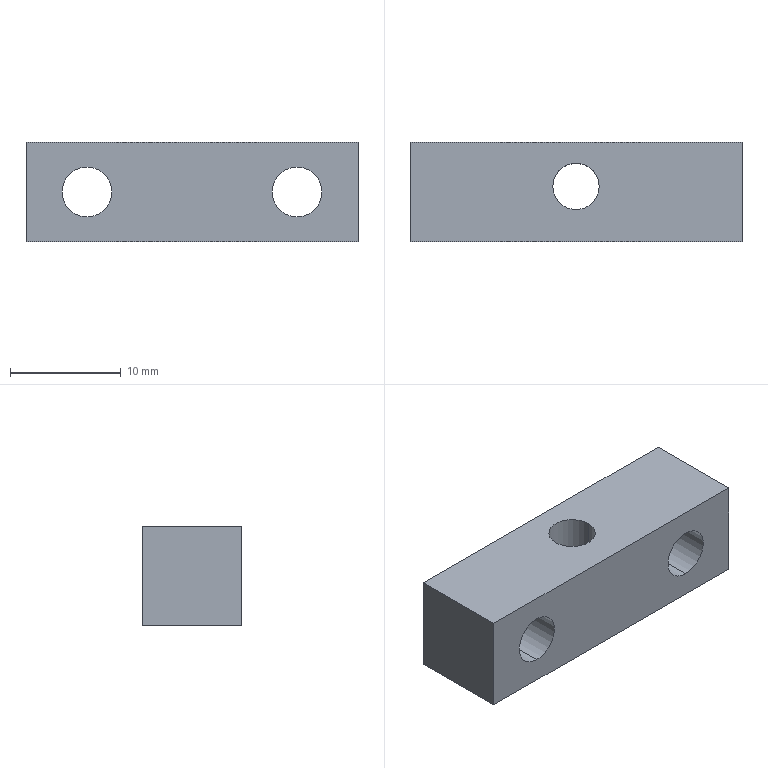Part | STEP file | SceondTSE6-8_Default | 1 solid | 18 faces | box 30 x 9 x 9 mm | volume 1675 mm3 | cylinder 10 | plane 8 | commonest cylinder face diameters 4.5 x4 8 x4 4.2 x2
STEP:
#1=CARTESIAN_POINT('',(0.,0.,0.));
#2=DIRECTION('',(0.,0.,1.));
#3=DIRECTION('',(1.,0.,0.));
#4=AXIS2_PLACEMENT_3D('',#1,#2,#3);
#5=CARTESIAN_POINT('',(2.1,5.,-4.5));
#6=VERTEX_POINT('',#5);
#7=CARTESIAN_POINT('',(2.1,5.,4.5));
#8=VERTEX_POINT('',#7);
#9=CARTESIAN_POINT('',(2.1,5.,4.5));
#10=DIRECTION('',(0.,0.,1.));
#11=VECTOR('',#10,1.);
#12=LINE('',#9,#11);
#13=CARTESIAN_POINT('',(0.,5.,4.5));
#14=DIRECTION('',(0.,0.,1.));
#15=DIRECTION('',(1.,0.,0.));
#16=AXIS2_PLACEMENT_3D('',#13,#14,#15);
#17=CYLINDRICAL_SURFACE('',#16,2.1);
#18=CARTESIAN_POINT('',(6.283,0.));
#19=DIRECTION('',(0.,1.));
#20=VECTOR('',#19,1.);
#21=LINE('',#18,#20);
#22=(GEOMETRIC_REPRESENTATION_CONTEXT(2)PARAMETRIC_REPRESENTATION_CONTEXT()REPRESENTATION_CONTEXT('',''));
#23=DEFINITIONAL_REPRESENTATION('',(#21),#22);
#24=PCURVE('',#17,#23);
#25=CARTESIAN_POINT('',(0.,5.,4.5));
#26=DIRECTION('',(0.,0.,1.));
#27=DIRECTION('',(1.,0.,0.));
#28=AXIS2_PLACEMENT_3D('',#25,#26,#27);
#29=CYLINDRICAL_SURFACE('',#28,2.1);
#30=CARTESIAN_POINT('',(0.,0.));
#31=DIRECTION('',(0.,1.));
#32=VECTOR('',#31,1.);
#33=LINE('',#30,#32);
#34=(GEOMETRIC_REPRESENTATION_CONTEXT(2)PARAMETRIC_REPRESENTATION_CONTEXT()REPRESENTATION_CONTEXT('',''));
#35=DEFINITIONAL_REPRESENTATION('',(#33),#34);
#36=PCURVE('',#29,#35);
#37=SURFACE_CURVE('',#12,(#24,#36),.PCURVE_S1.);
#38=EDGE_CURVE('',#6,#8,#37,.T.);
#39=ORIENTED_EDGE('',*,*,#38,.T.);
#40=CARTESIAN_POINT('',(-2.1,5.,4.5));
#41=VERTEX_POINT('',#40);
#42=CARTESIAN_POINT('',(0.,5.,4.5));
#43=DIRECTION('',(0.,0.,1.));
#44=DIRECTION('',(1.,0.,0.));
#45=AXIS2_PLACEMENT_3D('',#42,#43,#44);
#46=CIRCLE('',#45,2.1);
#47=CARTESIAN_POINT('',(0.,0.));
#48=DIRECTION('',(1.,0.));
#49=VECTOR('',#48,1.);
#50=LINE('',#47,#49);
#51=(GEOMETRIC_REPRESENTATION_CONTEXT(2)PARAMETRIC_REPRESENTATION_CONTEXT()REPRESENTATION_CONTEXT('',''));
#52=DEFINITIONAL_REPRESENTATION('',(#50),#51);
#53=PCURVE('',#17,#52);
#54=CARTESIAN_POINT('',(15.,9.,4.5));
#55=DIRECTION('',(0.,0.,-1.));
#56=DIRECTION('',(-1.,0.,0.));
#57=AXIS2_PLACEMENT_3D('',#54,#55,#56);
#58=PLANE('',#57);
#59=CARTESIAN_POINT('',(12.9,-4.));
#60=CARTESIAN_POINT('',(12.9,-0.3627));
#61=CARTESIAN_POINT('',(16.05,-2.181));
#62=CARTESIAN_POINT('',(19.2,-4.));
#63=CARTESIAN_POINT('',(16.05,-5.819));
#64=CARTESIAN_POINT('',(12.9,-7.637));
#65=CARTESIAN_POINT('',(12.9,-4.));
#66=(BOUNDED_CURVE()B_SPLINE_CURVE(2,(#59,#60,#61,#62,#63,#64,#65),.UNSPECIFIED.,.T.,.F.)B_SPLINE_CURVE_WITH_KNOTS((1,2,2,2,2,1),(-2.094,0.,2.094,4.189,6.283,8.378),.UNSPECIFIED.)CURVE()GEOMETRIC_REPRESENTATION_ITEM()RATIONAL_B_SPLINE_CURVE((1.,0.5,1.,0.5,1.,0.5,1.))REPRESENTATION_ITEM(''));
#67=(GEOMETRIC_REPRESENTATION_CONTEXT(2)PARAMETRIC_REPRESENTATION_CONTEXT()REPRESENTATION_CONTEXT('',''));
#68=DEFINITIONAL_REPRESENTATION('',(#66),#67);
#69=PCURVE('',#58,#68);
#70=SURFACE_CURVE('',#46,(#53,#69),.PCURVE_S1.);
#71=EDGE_CURVE('',#41,#8,#70,.T.);
#72=ORIENTED_EDGE('',*,*,#71,.F.);
#73=CARTESIAN_POINT('',(-2.1,5.,-4.5));
#74=VERTEX_POINT('',#73);
#75=CARTESIAN_POINT('',(-2.1,5.,4.5));
#76=DIRECTION('',(0.,0.,1.));
#77=VECTOR('',#76,1.);
#78=LINE('',#75,#77);
#79=CARTESIAN_POINT('',(3.142,0.));
#80=DIRECTION('',(0.,1.));
#81=VECTOR('',#80,1.);
#82=LINE('',#79,#81);
#83=(GEOMETRIC_REPRESENTATION_CONTEXT(2)PARAMETRIC_REPRESENTATION_CONTEXT()REPRESENTATION_CONTEXT('',''));
#84=DEFINITIONAL_REPRESENTATION('',(#82),#83);
#85=PCURVE('',#17,#84);
#86=CARTESIAN_POINT('',(3.142,0.));
#87=DIRECTION('',(0.,1.));
#88=VECTOR('',#87,1.);
#89=LINE('',#86,#88);
#90=(GEOMETRIC_REPRESENTATION_CONTEXT(2)PARAMETRIC_REPRESENTATION_CONTEXT()REPRESENTATION_CONTEXT('',''));
#91=DEFINITIONAL_REPRESENTATION('',(#89),#90);
#92=PCURVE('',#29,#91);
#93=SURFACE_CURVE('',#78,(#85,#92),.PCURVE_S1.);
#94=EDGE_CURVE('',#74,#41,#93,.T.);
#95=ORIENTED_EDGE('',*,*,#94,.F.);
#96=CARTESIAN_POINT('',(0.,5.,-4.5));
#97=DIRECTION('',(0.,0.,1.));
#98=DIRECTION('',(1.,0.,0.));
#99=AXIS2_PLACEMENT_3D('',#96,#97,#98);
#100=CIRCLE('',#99,2.1);
#101=CARTESIAN_POINT('',(0.,-9.));
#102=DIRECTION('',(1.,0.));
#103=VECTOR('',#102,1.);
#104=LINE('',#101,#103);
#105=(GEOMETRIC_REPRESENTATION_CONTEXT(2)PARAMETRIC_REPRESENTATION_CONTEXT()REPRESENTATION_CONTEXT('',''));
#106=DEFINITIONAL_REPRESENTATION('',(#104),#105);
#107=PCURVE('',#17,#106);
#108=CARTESIAN_POINT('',(15.,9.,-4.5));
#109=DIRECTION('',(0.,0.,1.));
#110=DIRECTION('',(1.,0.,0.));
#111=AXIS2_PLACEMENT_3D('',#108,#109,#110);
#112=PLANE('',#111);
#113=CARTESIAN_POINT('',(-15.,-4.));
#114=DIRECTION('',(1.,0.));
#115=AXIS2_PLACEMENT_2D('',#113,#114);
#116=CIRCLE('',#115,2.1);
#117=(GEOMETRIC_REPRESENTATION_CONTEXT(2)PARAMETRIC_REPRESENTATION_CONTEXT()REPRESENTATION_CONTEXT('',''));
#118=DEFINITIONAL_REPRESENTATION('',(#116),#117);
#119=PCURVE('',#112,#118);
#120=SURFACE_CURVE('',#100,(#107,#119),.PCURVE_S1.);
#121=EDGE_CURVE('',#74,#6,#120,.T.);
#122=ORIENTED_EDGE('',*,*,#121,.T.);
#123=EDGE_LOOP('',(#39,#72,#95,#122));
#124=FACE_BOUND('',#123,.F.);
#125=ADVANCED_FACE('',(#124),#17,.F.);
#126=CARTESIAN_POINT('',(-9.5,4.,4.));
#127=VERTEX_POINT('',#126);
#128=CARTESIAN_POINT('',(-9.5,9.,4.));
#129=VERTEX_POINT('',#128);
#130=CARTESIAN_POINT('',(-9.5,9.,4.));
#131=DIRECTION('',(0.,1.,0.));
#132=VECTOR('',#131,1.);
#133=LINE('',#130,#132);
#134=CARTESIAN_POINT('',(-9.5,9.,0.));
#135=DIRECTION('',(0.,1.,0.));
#136=DIRECTION('',(0.,0.,1.));
#137=AXIS2_PLACEMENT_3D('',#134,#135,#136);
#138=CYLINDRICAL_SURFACE('',#137,4.);
#139=CARTESIAN_POINT('',(6.283,0.));
#140=DIRECTION('',(0.,1.));
#141=VECTOR('',#140,1.);
#142=LINE('',#139,#141);
#143=(GEOMETRIC_REPRESENTATION_CONTEXT(2)PARAMETRIC_REPRESENTATION_CONTEXT()REPRESENTATION_CONTEXT('',''));
#144=DEFINITIONAL_REPRESENTATION('',(#142),#143);
#145=PCURVE('',#138,#144);
#146=CARTESIAN_POINT('',(-9.5,9.,0.));
#147=DIRECTION('',(0.,1.,0.));
#148=DIRECTION('',(0.,0.,1.));
#149=AXIS2_PLACEMENT_3D('',#146,#147,#148);
#150=CYLINDRICAL_SURFACE('',#149,4.);
#151=CARTESIAN_POINT('',(0.,0.));
#152=DIRECTION('',(0.,1.));
#153=VECTOR('',#152,1.);
#154=LINE('',#151,#153);
#155=(GEOMETRIC_REPRESENTATION_CONTEXT(2)PARAMETRIC_REPRESENTATION_CONTEXT()REPRESENTATION_CONTEXT('',''));
#156=DEFINITIONAL_REPRESENTATION('',(#154),#155);
#157=PCURVE('',#150,#156);
#158=SURFACE_CURVE('',#133,(#145,#157),.PCURVE_S1.);
#159=EDGE_CURVE('',#127,#129,#158,.T.);
#160=ORIENTED_EDGE('',*,*,#159,.T.);
#161=CARTESIAN_POINT('',(-9.5,9.,-4.));
#162=VERTEX_POINT('',#161);
#163=CARTESIAN_POINT('',(-9.5,9.,0.));
#164=DIRECTION('',(0.,1.,0.));
#165=DIRECTION('',(0.,0.,1.));
#166=AXIS2_PLACEMENT_3D('',#163,#164,#165);
#167=CIRCLE('',#166,4.);
#168=CARTESIAN_POINT('',(0.,0.));
#169=DIRECTION('',(1.,0.));
#170=VECTOR('',#169,1.);
#171=LINE('',#168,#170);
#172=(GEOMETRIC_REPRESENTATION_CONTEXT(2)PARAMETRIC_REPRESENTATION_CONTEXT()REPRESENTATION_CONTEXT('',''));
#173=DEFINITIONAL_REPRESENTATION('',(#171),#172);
#174=PCURVE('',#138,#173);
#175=CARTESIAN_POINT('',(0.,9.,0.));
#176=DIRECTION('',(0.,1.,0.));
#177=DIRECTION('',(0.,0.,1.));
#178=AXIS2_PLACEMENT_3D('',#175,#176,#177);
#179=PLANE('',#178);
#180=CARTESIAN_POINT('',(0.,-9.5));
#181=DIRECTION('',(1.,0.));
#182=AXIS2_PLACEMENT_2D('',#180,#181);
#183=CIRCLE('',#182,4.);
#184=(GEOMETRIC_REPRESENTATION_CONTEXT(2)PARAMETRIC_REPRESENTATION_CONTEXT()REPRESENTATION_CONTEXT('',''));
#185=DEFINITIONAL_REPRESENTATION('',(#183),#184);
#186=PCURVE('',#179,#185);
#187=SURFACE_CURVE('',#167,(#174,#186),.PCURVE_S1.);
#188=EDGE_CURVE('',#162,#129,#187,.T.);
#189=ORIENTED_EDGE('',*,*,#188,.F.);
#190=CARTESIAN_POINT('',(-9.5,4.,-4.));
#191=VERTEX_POINT('',#190);
#192=CARTESIAN_POINT('',(-9.5,9.,-4.));
#193=DIRECTION('',(0.,1.,0.));
#194=VECTOR('',#193,1.);
#195=LINE('',#192,#194);
#196=CARTESIAN_POINT('',(3.142,0.));
#197=DIRECTION('',(0.,1.));
#198=VECTOR('',#197,1.);
#199=LINE('',#196,#198);
#200=(GEOMETRIC_REPRESENTATION_CONTEXT(2)PARAMETRIC_REPRESENTATION_CONTEXT()REPRESENTATION_CONTEXT('',''));
#201=DEFINITIONAL_REPRESENTATION('',(#199),#200);
#202=PCURVE('',#138,#201);
#203=CARTESIAN_POINT('',(3.142,0.));
#204=DIRECTION('',(0.,1.));
#205=VECTOR('',#204,1.);
#206=LINE('',#203,#205);
#207=(GEOMETRIC_REPRESENTATION_CONTEXT(2)PARAMETRIC_REPRESENTATION_CONTEXT()REPRESENTATION_CONTEXT('',''));
#208=DEFINITIONAL_REPRESENTATION('',(#206),#207);
#209=PCURVE('',#150,#208);
#210=SURFACE_CURVE('',#195,(#202,#209),.PCURVE_S1.);
#211=EDGE_CURVE('',#191,#162,#210,.T.);
#212=ORIENTED_EDGE('',*,*,#211,.F.);
#213=CARTESIAN_POINT('',(-9.5,4.,0.));
#214=DIRECTION('',(0.,1.,0.));
#215=DIRECTION('',(0.,0.,1.));
#216=AXIS2_PLACEMENT_3D('',#213,#214,#215);
#217=CIRCLE('',#216,4.);
#218=CARTESIAN_POINT('',(0.,-5.));
#219=DIRECTION('',(1.,0.));
#220=VECTOR('',#219,1.);
#221=LINE('',#218,#220);
#222=(GEOMETRIC_REPRESENTATION_CONTEXT(2)PARAMETRIC_REPRESENTATION_CONTEXT()REPRESENTATION_CONTEXT('',''));
#223=DEFINITIONAL_REPRESENTATION('',(#221),#222);
#224=PCURVE('',#138,#223);
#225=CARTESIAN_POINT('',(-7.25,4.,0.));
#226=DIRECTION('',(0.,-1.,0.));
#227=DIRECTION('',(0.,0.,-1.));
#228=AXIS2_PLACEMENT_3D('',#225,#226,#227);
#229=PLANE('',#228);
#230=CARTESIAN_POINT('',(-4.,-2.25));
#231=CARTESIAN_POINT('',(-4.,4.678));
#232=CARTESIAN_POINT('',(2.,1.214));
#233=CARTESIAN_POINT('',(8.,-2.25));
#234=CARTESIAN_POINT('',(2.,-5.714));
#235=CARTESIAN_POINT('',(-4.,-9.178));
#236=CARTESIAN_POINT('',(-4.,-2.25));
#237=(BOUNDED_CURVE()B_SPLINE_CURVE(2,(#230,#231,#232,#233,#234,#235,#236),.UNSPECIFIED.,.T.,.F.)B_SPLINE_CURVE_WITH_KNOTS((1,2,2,2,2,1),(-2.094,0.,2.094,4.189,6.283,8.378),.UNSPECIFIED.)CURVE()GEOMETRIC_REPRESENTATION_ITEM()RATIONAL_B_SPLINE_CURVE((1.,0.5,1.,0.5,1.,0.5,1.))REPRESENTATION_ITEM(''));
#238=(GEOMETRIC_REPRESENTATION_CONTEXT(2)PARAMETRIC_REPRESENTATION_CONTEXT()REPRESENTATION_CONTEXT('',''));
#239=DEFINITIONAL_REPRESENTATION('',(#237),#238);
#240=PCURVE('',#229,#239);
#241=SURFACE_CURVE('',#217,(#224,#240),.PCURVE_S1.);
#242=EDGE_CURVE('',#191,#127,#241,.T.);
#243=ORIENTED_EDGE('',*,*,#242,.T.);
#244=EDGE_LOOP('',(#160,#189,#212,#243));
#245=FACE_BOUND('',#244,.F.);
#246=ADVANCED_FACE('',(#245),#138,.F.);
#247=CARTESIAN_POINT('',(-9.5,0.,2.25));
#248=VERTEX_POINT('',#247);
#249=CARTESIAN_POINT('',(-9.5,4.,2.25));
#250=VERTEX_POINT('',#249);
#251=CARTESIAN_POINT('',(-9.5,9.,2.25));
#252=DIRECTION('',(0.,1.,0.));
#253=VECTOR('',#252,1.);
#254=LINE('',#251,#253);
#255=CARTESIAN_POINT('',(-9.5,9.,0.));
#256=DIRECTION('',(0.,1.,0.));
#257=DIRECTION('',(0.,0.,1.));
#258=AXIS2_PLACEMENT_3D('',#255,#256,#257);
#259=CYLINDRICAL_SURFACE('',#258,2.25);
#260=CARTESIAN_POINT('',(6.283,0.));
#261=DIRECTION('',(0.,1.));
#262=VECTOR('',#261,1.);
#263=LINE('',#260,#262);
#264=(GEOMETRIC_REPRESENTATION_CONTEXT(2)PARAMETRIC_REPRESENTATION_CONTEXT()REPRESENTATION_CONTEXT('',''));
#265=DEFINITIONAL_REPRESENTATION('',(#263),#264);
#266=PCURVE('',#259,#265);
#267=CARTESIAN_POINT('',(-9.5,9.,0.));
#268=DIRECTION('',(0.,1.,0.));
#269=DIRECTION('',(0.,0.,1.));
#270=AXIS2_PLACEMENT_3D('',#267,#268,#269);
#271=CYLINDRICAL_SURFACE('',#270,2.25);
#272=CARTESIAN_POINT('',(0.,0.));
#273=DIRECTION('',(0.,1.));
#274=VECTOR('',#273,1.);
#275=LINE('',#272,#274);
#276=(GEOMETRIC_REPRESENTATION_CONTEXT(2)PARAMETRIC_REPRESENTATION_CONTEXT()REPRESENTATION_CONTEXT('',''));
#277=DEFINITIONAL_REPRESENTATION('',(#275),#276);
#278=PCURVE('',#271,#277);
#279=SURFACE_CURVE('',#254,(#266,#278),.PCURVE_S1.);
#280=EDGE_CURVE('',#248,#250,#279,.T.);
#281=ORIENTED_EDGE('',*,*,#280,.T.);
#282=CARTESIAN_POINT('',(-9.5,4.,-2.25));
#283=VERTEX_POINT('',#282);
#284=CARTESIAN_POINT('',(-9.5,4.,0.));
#285=DIRECTION('',(0.,1.,0.));
#286=DIRECTION('',(0.,0.,1.));
#287=AXIS2_PLACEMENT_3D('',#284,#285,#286);
#288=CIRCLE('',#287,2.25);
#289=CARTESIAN_POINT('',(0.,-5.));
#290=DIRECTION('',(1.,0.));
#291=VECTOR('',#290,1.);
#292=LINE('',#289,#291);
#293=(GEOMETRIC_REPRESENTATION_CONTEXT(2)PARAMETRIC_REPRESENTATION_CONTEXT()REPRESENTATION_CONTEXT('',''));
#294=DEFINITIONAL_REPRESENTATION('',(#292),#293);
#295=PCURVE('',#259,#294);
#296=CARTESIAN_POINT('',(-2.25,-2.25));
#297=CARTESIAN_POINT('',(-2.25,1.647));
#298=CARTESIAN_POINT('',(1.125,-0.3014));
#299=CARTESIAN_POINT('',(4.5,-2.25));
#300=CARTESIAN_POINT('',(1.125,-4.199));
#301=CARTESIAN_POINT('',(-2.25,-6.147));
#302=CARTESIAN_POINT('',(-2.25,-2.25));
#303=(BOUNDED_CURVE()B_SPLINE_CURVE(2,(#296,#297,#298,#299,#300,#301,#302),.UNSPECIFIED.,.T.,.F.)B_SPLINE_CURVE_WITH_KNOTS((1,2,2,2,2,1),(-2.094,0.,2.094,4.189,6.283,8.378),.UNSPECIFIED.)CURVE()GEOMETRIC_REPRESENTATION_ITEM()RATIONAL_B_SPLINE_CURVE((1.,0.5,1.,0.5,1.,0.5,1.))REPRESENTATION_ITEM(''));
#304=(GEOMETRIC_REPRESENTATION_CONTEXT(2)PARAMETRIC_REPRESENTATION_CONTEXT()REPRESENTATION_CONTEXT('',''));
#305=DEFINITIONAL_REPRESENTATION('',(#303),#304);
#306=PCURVE('',#229,#305);
#307=SURFACE_CURVE('',#288,(#295,#306),.PCURVE_S1.);
#308=EDGE_CURVE('',#283,#250,#307,.T.);
#309=ORIENTED_EDGE('',*,*,#308,.F.);
#310=CARTESIAN_POINT('',(-9.5,0.,-2.25));
#311=VERTEX_POINT('',#310);
#312=CARTESIAN_POINT('',(-9.5,9.,-2.25));
#313=DIRECTION('',(0.,1.,0.));
#314=VECTOR('',#313,1.);
#315=LINE('',#312,#314);
#316=CARTESIAN_POINT('',(3.142,0.));
#317=DIRECTION('',(0.,1.));
#318=VECTOR('',#317,1.);
#319=LINE('',#316,#318);
#320=(GEOMETRIC_REPRESENTATION_CONTEXT(2)PARAMETRIC_REPRESENTATION_CONTEXT()REPRESENTATION_CONTEXT('',''));
#321=DEFINITIONAL_REPRESENTATION('',(#319),#320);
#322=PCURVE('',#259,#321);
#323=CARTESIAN_POINT('',(3.142,0.));
#324=DIRECTION('',(0.,1.));
#325=VECTOR('',#324,1.);
#326=LINE('',#323,#325);
#327=(GEOMETRIC_REPRESENTATION_CONTEXT(2)PARAMETRIC_REPRESENTATION_CONTEXT()REPRESENTATION_CONTEXT('',''));
#328=DEFINITIONAL_REPRESENTATION('',(#326),#327);
#329=PCURVE('',#271,#328);
#330=SURFACE_CURVE('',#315,(#322,#329),.PCURVE_S1.);
#331=EDGE_CURVE('',#311,#283,#330,.T.);
#332=ORIENTED_EDGE('',*,*,#331,.F.);
#333=CARTESIAN_POINT('',(-9.5,0.,0.));
#334=DIRECTION('',(0.,1.,0.));
#335=DIRECTION('',(0.,0.,1.));
#336=AXIS2_PLACEMENT_3D('',#333,#334,#335);
#337=CIRCLE('',#336,2.25);
#338=CARTESIAN_POINT('',(0.,-9.));
#339=DIRECTION('',(1.,0.));
#340=VECTOR('',#339,1.);
#341=LINE('',#338,#340);
#342=(GEOMETRIC_REPRESENTATION_CONTEXT(2)PARAMETRIC_REPRESENTATION_CONTEXT()REPRESENTATION_CONTEXT('',''));
#343=DEFINITIONAL_REPRESENTATION('',(#341),#342);
#344=PCURVE('',#259,#343);
#345=CARTESIAN_POINT('',(0.,0.,0.));
#346=DIRECTION('',(0.,1.,0.));
#347=DIRECTION('',(0.,0.,1.));
#348=AXIS2_PLACEMENT_3D('',#345,#346,#347);
#349=PLANE('',#348);
#350=CARTESIAN_POINT('',(0.,-9.5));
#351=DIRECTION('',(1.,0.));
#352=AXIS2_PLACEMENT_2D('',#350,#351);
#353=CIRCLE('',#352,2.25);
#354=(GEOMETRIC_REPRESENTATION_CONTEXT(2)PARAMETRIC_REPRESENTATION_CONTEXT()REPRESENTATION_CONTEXT('',''));
#355=DEFINITIONAL_REPRESENTATION('',(#353),#354);
#356=PCURVE('',#349,#355);
#357=SURFACE_CURVE('',#337,(#344,#356),.PCURVE_S1.);
#358=EDGE_CURVE('',#311,#248,#357,.T.);
#359=ORIENTED_EDGE('',*,*,#358,.T.);
#360=EDGE_LOOP('',(#281,#309,#332,#359));
#361=FACE_BOUND('',#360,.F.);
#362=ADVANCED_FACE('',(#361),#259,.F.);
#363=CARTESIAN_POINT('',(9.5,4.,4.));
#364=VERTEX_POINT('',#363);
#365=CARTESIAN_POINT('',(9.5,9.,4.));
#366=VERTEX_POINT('',#365);
#367=CARTESIAN_POINT('',(9.5,9.,4.));
#368=DIRECTION('',(0.,1.,0.));
#369=VECTOR('',#368,1.);
#370=LINE('',#367,#369);
#371=CARTESIAN_POINT('',(9.5,9.,0.));
#372=DIRECTION('',(0.,1.,0.));
#373=DIRECTION('',(0.,0.,1.));
#374=AXIS2_PLACEMENT_3D('',#371,#372,#373);
#375=CYLINDRICAL_SURFACE('',#374,4.);
#376=CARTESIAN_POINT('',(6.283,0.));
#377=DIRECTION('',(0.,1.));
#378=VECTOR('',#377,1.);
#379=LINE('',#376,#378);
#380=(GEOMETRIC_REPRESENTATION_CONTEXT(2)PARAMETRIC_REPRESENTATION_CONTEXT()REPRESENTATION_CONTEXT('',''));
#381=DEFINITIONAL_REPRESENTATION('',(#379),#380);
#382=PCURVE('',#375,#381);
#383=CARTESIAN_POINT('',(9.5,9.,0.));
#384=DIRECTION('',(0.,1.,0.));
#385=DIRECTION('',(0.,0.,1.));
#386=AXIS2_PLACEMENT_3D('',#383,#384,#385);
#387=CYLINDRICAL_SURFACE('',#386,4.);
#388=CARTESIAN_POINT('',(0.,0.));
#389=DIRECTION('',(0.,1.));
#390=VECTOR('',#389,1.);
#391=LINE('',#388,#390);
#392=(GEOMETRIC_REPRESENTATION_CONTEXT(2)PARAMETRIC_REPRESENTATION_CONTEXT()REPRESENTATION_CONTEXT('',''));
#393=DEFINITIONAL_REPRESENTATION('',(#391),#392);
#394=PCURVE('',#387,#393);
#395=SURFACE_CURVE('',#370,(#382,#394),.PCURVE_S1.);
#396=EDGE_CURVE('',#364,#366,#395,.T.);
#397=ORIENTED_EDGE('',*,*,#396,.T.);
#398=CARTESIAN_POINT('',(9.5,9.,-4.));
#399=VERTEX_POINT('',#398);
#400=CARTESIAN_POINT('',(9.5,9.,0.));
#401=DIRECTION('',(0.,1.,0.));
#402=DIRECTION('',(0.,0.,1.));
#403=AXIS2_PLACEMENT_3D('',#400,#401,#402);
#404=CIRCLE('',#403,4.);
#405=CARTESIAN_POINT('',(0.,0.));
#406=DIRECTION('',(1.,0.));
#407=VECTOR('',#406,1.);
#408=LINE('',#405,#407);
#409=(GEOMETRIC_REPRESENTATION_CONTEXT(2)PARAMETRIC_REPRESENTATION_CONTEXT()REPRESENTATION_CONTEXT('',''));
#410=DEFINITIONAL_REPRESENTATION('',(#408),#409);
#411=PCURVE('',#375,#410);
#412=CARTESIAN_POINT('',(0.,9.5));
#413=DIRECTION('',(1.,0.));
#414=AXIS2_PLACEMENT_2D('',#412,#413);
#415=CIRCLE('',#414,4.);
#416=(GEOMETRIC_REPRESENTATION_CONTEXT(2)PARAMETRIC_REPRESENTATION_CONTEXT()REPRESENTATION_CONTEXT('',''));
#417=DEFINITIONAL_REPRESENTATION('',(#415),#416);
#418=PCURVE('',#179,#417);
#419=SURFACE_CURVE('',#404,(#411,#418),.PCURVE_S1.);
#420=EDGE_CURVE('',#399,#366,#419,.T.);
#421=ORIENTED_EDGE('',*,*,#420,.F.);
#422=CARTESIAN_POINT('',(9.5,4.,-4.));
#423=VERTEX_POINT('',#422);
#424=CARTESIAN_POINT('',(9.5,9.,-4.));
#425=DIRECTION('',(0.,1.,0.));
#426=VECTOR('',#425,1.);
#427=LINE('',#424,#426);
#428=CARTESIAN_POINT('',(3.142,0.));
#429=DIRECTION('',(0.,1.));
#430=VECTOR('',#429,1.);
#431=LINE('',#428,#430);
#432=(GEOMETRIC_REPRESENTATION_CONTEXT(2)PARAMETRIC_REPRESENTATION_CONTEXT()REPRESENTATION_CONTEXT('',''));
#433=DEFINITIONAL_REPRESENTATION('',(#431),#432);
#434=PCURVE('',#375,#433);
#435=CARTESIAN_POINT('',(3.142,0.));
#436=DIRECTION('',(0.,1.));
#437=VECTOR('',#436,1.);
#438=LINE('',#435,#437);
#439=(GEOMETRIC_REPRESENTATION_CONTEXT(2)PARAMETRIC_REPRESENTATION_CONTEXT()REPRESENTATION_CONTEXT('',''));
#440=DEFINITIONAL_REPRESENTATION('',(#438),#439);
#441=PCURVE('',#387,#440);
#442=SURFACE_CURVE('',#427,(#434,#441),.PCURVE_S1.);
#443=EDGE_CURVE('',#423,#399,#442,.T.);
#444=ORIENTED_EDGE('',*,*,#443,.F.);
#445=CARTESIAN_POINT('',(9.5,4.,0.));
#446=DIRECTION('',(0.,1.,0.));
#447=DIRECTION('',(0.,0.,1.));
#448=AXIS2_PLACEMENT_3D('',#445,#446,#447);
#449=CIRCLE('',#448,4.);
#450=CARTESIAN_POINT('',(0.,-5.));
#451=DIRECTION('',(1.,0.));
#452=VECTOR('',#451,1.);
#453=LINE('',#450,#452);
#454=(GEOMETRIC_REPRESENTATION_CONTEXT(2)PARAMETRIC_REPRESENTATION_CONTEXT()REPRESENTATION_CONTEXT('',''));
#455=DEFINITIONAL_REPRESENTATION('',(#453),#454);
#456=PCURVE('',#375,#455);
#457=CARTESIAN_POINT('',(11.75,4.,0.));
#458=DIRECTION('',(0.,-1.,0.));
#459=DIRECTION('',(0.,0.,-1.));
#460=AXIS2_PLACEMENT_3D('',#457,#458,#459);
#461=PLANE('',#460);
#462=CARTESIAN_POINT('',(-4.,-2.25));
#463=CARTESIAN_POINT('',(-4.,4.678));
#464=CARTESIAN_POINT('',(2.,1.214));
#465=CARTESIAN_POINT('',(8.,-2.25));
#466=CARTESIAN_POINT('',(2.,-5.714));
#467=CARTESIAN_POINT('',(-4.,-9.178));
#468=CARTESIAN_POINT('',(-4.,-2.25));
#469=(BOUNDED_CURVE()B_SPLINE_CURVE(2,(#462,#463,#464,#465,#466,#467,#468),.UNSPECIFIED.,.T.,.F.)B_SPLINE_CURVE_WITH_KNOTS((1,2,2,2,2,1),(-2.094,0.,2.094,4.189,6.283,8.378),.UNSPECIFIED.)CURVE()GEOMETRIC_REPRESENTATION_ITEM()RATIONAL_B_SPLINE_CURVE((1.,0.5,1.,0.5,1.,0.5,1.))REPRESENTATION_ITEM(''));
#470=(GEOMETRIC_REPRESENTATION_CONTEXT(2)PARAMETRIC_REPRESENTATION_CONTEXT()REPRESENTATION_CONTEXT('',''));
#471=DEFINITIONAL_REPRESENTATION('',(#469),#470);
#472=PCURVE('',#461,#471);
#473=SURFACE_CURVE('',#449,(#456,#472),.PCURVE_S1.);
#474=EDGE_CURVE('',#423,#364,#473,.T.);
#475=ORIENTED_EDGE('',*,*,#474,.T.);
#476=EDGE_LOOP('',(#397,#421,#444,#475));
#477=FACE_BOUND('',#476,.F.);
#478=ADVANCED_FACE('',(#477),#375,.F.);
#479=CARTESIAN_POINT('',(9.5,0.,2.25));
#480=VERTEX_POINT('',#479);
#481=CARTESIAN_POINT('',(9.5,4.,2.25));
#482=VERTEX_POINT('',#481);
#483=CARTESIAN_POINT('',(9.5,9.,2.25));
#484=DIRECTION('',(0.,1.,0.));
#485=VECTOR('',#484,1.);
#486=LINE('',#483,#485);
#487=CARTESIAN_POINT('',(9.5,9.,0.));
#488=DIRECTION('',(0.,1.,0.));
#489=DIRECTION('',(0.,0.,1.));
#490=AXIS2_PLACEMENT_3D('',#487,#488,#489);
#491=CYLINDRICAL_SURFACE('',#490,2.25);
#492=CARTESIAN_POINT('',(6.283,0.));
#493=DIRECTION('',(0.,1.));
#494=VECTOR('',#493,1.);
#495=LINE('',#492,#494);
#496=(GEOMETRIC_REPRESENTATION_CONTEXT(2)PARAMETRIC_REPRESENTATION_CONTEXT()REPRESENTATION_CONTEXT('',''));
#497=DEFINITIONAL_REPRESENTATION('',(#495),#496);
#498=PCURVE('',#491,#497);
#499=CARTESIAN_POINT('',(9.5,9.,0.));
#500=DIRECTION('',(0.,1.,0.));
#501=DIRECTION('',(0.,0.,1.));
#502=AXIS2_PLACEMENT_3D('',#499,#500,#501);
#503=CYLINDRICAL_SURFACE('',#502,2.25);
#504=CARTESIAN_POINT('',(0.,0.));
#505=DIRECTION('',(0.,1.));
#506=VECTOR('',#505,1.);
#507=LINE('',#504,#506);
#508=(GEOMETRIC_REPRESENTATION_CONTEXT(2)PARAMETRIC_REPRESENTATION_CONTEXT()REPRESENTATION_CONTEXT('',''));
#509=DEFINITIONAL_REPRESENTATION('',(#507),#508);
#510=PCURVE('',#503,#509);
#511=SURFACE_CURVE('',#486,(#498,#510),.PCURVE_S1.);
#512=EDGE_CURVE('',#480,#482,#511,.T.);
#513=ORIENTED_EDGE('',*,*,#512,.T.);
#514=CARTESIAN_POINT('',(9.5,4.,-2.25));
#515=VERTEX_POINT('',#514);
#516=CARTESIAN_POINT('',(9.5,4.,0.));
#517=DIRECTION('',(0.,1.,0.));
#518=DIRECTION('',(0.,0.,1.));
#519=AXIS2_PLACEMENT_3D('',#516,#517,#518);
#520=CIRCLE('',#519,2.25);
#521=CARTESIAN_POINT('',(0.,-5.));
#522=DIRECTION('',(1.,0.));
#523=VECTOR('',#522,1.);
#524=LINE('',#521,#523);
#525=(GEOMETRIC_REPRESENTATION_CONTEXT(2)PARAMETRIC_REPRESENTATION_CONTEXT()REPRESENTATION_CONTEXT('',''));
#526=DEFINITIONAL_REPRESENTATION('',(#524),#525);
#527=PCURVE('',#491,#526);
#528=CARTESIAN_POINT('',(-2.25,-2.25));
#529=CARTESIAN_POINT('',(-2.25,1.647));
#530=CARTESIAN_POINT('',(1.125,-0.3014));
#531=CARTESIAN_POINT('',(4.5,-2.25));
#532=CARTESIAN_POINT('',(1.125,-4.199));
#533=CARTESIAN_POINT('',(-2.25,-6.147));
#534=CARTESIAN_POINT('',(-2.25,-2.25));
#535=(BOUNDED_CURVE()B_SPLINE_CURVE(2,(#528,#529,#530,#531,#532,#533,#534),.UNSPECIFIED.,.T.,.F.)B_SPLINE_CURVE_WITH_KNOTS((1,2,2,2,2,1),(-2.094,0.,2.094,4.189,6.283,8.378),.UNSPECIFIED.)CURVE()GEOMETRIC_REPRESENTATION_ITEM()RATIONAL_B_SPLINE_CURVE((1.,0.5,1.,0.5,1.,0.5,1.))REPRESENTATION_ITEM(''));
#536=(GEOMETRIC_REPRESENTATION_CONTEXT(2)PARAMETRIC_REPRESENTATION_CONTEXT()REPRESENTATION_CONTEXT('',''));
#537=DEFINITIONAL_REPRESENTATION('',(#535),#536);
#538=PCURVE('',#461,#537);
#539=SURFACE_CURVE('',#520,(#527,#538),.PCURVE_S1.);
#540=EDGE_CURVE('',#515,#482,#539,.T.);
#541=ORIENTED_EDGE('',*,*,#540,.F.);
#542=CARTESIAN_POINT('',(9.5,0.,-2.25));
#543=VERTEX_POINT('',#542);
#544=CARTESIAN_POINT('',(9.5,9.,-2.25));
#545=DIRECTION('',(0.,1.,0.));
#546=VECTOR('',#545,1.);
#547=LINE('',#544,#546);
#548=CARTESIAN_POINT('',(3.142,0.));
#549=DIRECTION('',(0.,1.));
#550=VECTOR('',#549,1.);
#551=LINE('',#548,#550);
#552=(GEOMETRIC_REPRESENTATION_CONTEXT(2)PARAMETRIC_REPRESENTATION_CONTEXT()REPRESENTATION_CONTEXT('',''));
#553=DEFINITIONAL_REPRESENTATION('',(#551),#552);
#554=PCURVE('',#491,#553);
#555=CARTESIAN_POINT('',(3.142,0.));
#556=DIRECTION('',(0.,1.));
#557=VECTOR('',#556,1.);
#558=LINE('',#555,#557);
#559=(GEOMETRIC_REPRESENTATION_CONTEXT(2)PARAMETRIC_REPRESENTATION_CONTEXT()REPRESENTATION_CONTEXT('',''));
#560=DEFINITIONAL_REPRESENTATION('',(#558),#559);
#561=PCURVE('',#503,#560);
#562=SURFACE_CURVE('',#547,(#554,#561),.PCURVE_S1.);
#563=EDGE_CURVE('',#543,#515,#562,.T.);
#564=ORIENTED_EDGE('',*,*,#563,.F.);
#565=CARTESIAN_POINT('',(9.5,0.,0.));
#566=DIRECTION('',(0.,1.,0.));
#567=DIRECTION('',(0.,0.,1.));
#568=AXIS2_PLACEMENT_3D('',#565,#566,#567);
#569=CIRCLE('',#568,2.25);
#570=CARTESIAN_POINT('',(0.,-9.));
#571=DIRECTION('',(1.,0.));
#572=VECTOR('',#571,1.);
#573=LINE('',#570,#572);
#574=(GEOMETRIC_REPRESENTATION_CONTEXT(2)PARAMETRIC_REPRESENTATION_CONTEXT()REPRESENTATION_CONTEXT('',''));
#575=DEFINITIONAL_REPRESENTATION('',(#573),#574);
#576=PCURVE('',#491,#575);
#577=CARTESIAN_POINT('',(0.,9.5));
#578=DIRECTION('',(1.,0.));
#579=AXIS2_PLACEMENT_2D('',#577,#578);
#580=CIRCLE('',#579,2.25);
#581=(GEOMETRIC_REPRESENTATION_CONTEXT(2)PARAMETRIC_REPRESENTATION_CONTEXT()REPRESENTATION_CONTEXT('',''));
#582=DEFINITIONAL_REPRESENTATION('',(#580),#581);
#583=PCURVE('',#349,#582);
#584=SURFACE_CURVE('',#569,(#576,#583),.PCURVE_S1.);
#585=EDGE_CURVE('',#543,#480,#584,.T.);
#586=ORIENTED_EDGE('',*,*,#585,.T.);
#587=EDGE_LOOP('',(#513,#541,#564,#586));
#588=FACE_BOUND('',#587,.F.);
#589=ADVANCED_FACE('',(#588),#491,.F.);
#590=CARTESIAN_POINT('',(-15.,0.,-4.5));
#591=VERTEX_POINT('',#590);
#592=CARTESIAN_POINT('',(-15.,0.,4.5));
#593=VERTEX_POINT('',#592);
#594=CARTESIAN_POINT('',(-15.,0.,4.5));
#595=DIRECTION('',(0.,0.,1.));
#596=VECTOR('',#595,1.);
#597=LINE('',#594,#596);
#598=CARTESIAN_POINT('',(-15.,9.,4.5));
#599=DIRECTION('',(1.,0.,0.));
#600=DIRECTION('',(0.,0.,-1.));
#601=AXIS2_PLACEMENT_3D('',#598,#599,#600);
#602=PLANE('',#601);
#603=CARTESIAN_POINT('',(0.,-9.));
#604=DIRECTION('',(-1.,0.));
#605=VECTOR('',#604,1.);
#606=LINE('',#603,#605);
#607=(GEOMETRIC_REPRESENTATION_CONTEXT(2)PARAMETRIC_REPRESENTATION_CONTEXT()REPRESENTATION_CONTEXT('',''));
#608=DEFINITIONAL_REPRESENTATION('',(#606),#607);
#609=PCURVE('',#602,#608);
#610=CARTESIAN_POINT('',(4.5,-15.));
#611=DIRECTION('',(1.,0.));
#612=VECTOR('',#611,1.);
#613=LINE('',#610,#612);
#614=(GEOMETRIC_REPRESENTATION_CONTEXT(2)PARAMETRIC_REPRESENTATION_CONTEXT()REPRESENTATION_CONTEXT('',''));
#615=DEFINITIONAL_REPRESENTATION('',(#613),#614);
#616=PCURVE('',#349,#615);
#617=SURFACE_CURVE('',#597,(#609,#616),.PCURVE_S1.);
#618=EDGE_CURVE('',#591,#593,#617,.T.);
#619=ORIENTED_EDGE('',*,*,#618,.T.);
#620=CARTESIAN_POINT('',(-15.,9.,4.5));
#621=VERTEX_POINT('',#620);
#622=CARTESIAN_POINT('',(-15.,9.,4.5));
#623=DIRECTION('',(0.,-1.,0.));
#624=VECTOR('',#623,1.);
#625=LINE('',#622,#624);
#626=CARTESIAN_POINT('',(0.,0.));
#627=DIRECTION('',(0.,-1.));
#628=VECTOR('',#627,1.);
#629=LINE('',#626,#628);
#630=(GEOMETRIC_REPRESENTATION_CONTEXT(2)PARAMETRIC_REPRESENTATION_CONTEXT()REPRESENTATION_CONTEXT('',''));
#631=DEFINITIONAL_REPRESENTATION('',(#629),#630);
#632=PCURVE('',#602,#631);
#633=CARTESIAN_POINT('',(30.,0.));
#634=DIRECTION('',(0.,-1.));
#635=VECTOR('',#634,1.);
#636=LINE('',#633,#635);
#637=(GEOMETRIC_REPRESENTATION_CONTEXT(2)PARAMETRIC_REPRESENTATION_CONTEXT()REPRESENTATION_CONTEXT('',''));
#638=DEFINITIONAL_REPRESENTATION('',(#636),#637);
#639=PCURVE('',#58,#638);
#640=SURFACE_CURVE('',#625,(#632,#639),.PCURVE_S1.);
#641=EDGE_CURVE('',#621,#593,#640,.T.);
#642=ORIENTED_EDGE('',*,*,#641,.F.);
#643=CARTESIAN_POINT('',(-15.,9.,-4.5));
#644=VERTEX_POINT('',#643);
#645=CARTESIAN_POINT('',(-15.,9.,4.5));
#646=DIRECTION('',(0.,0.,1.));
#647=VECTOR('',#646,1.);
#648=LINE('',#645,#647);
#649=CARTESIAN_POINT('',(0.,0.));
#650=DIRECTION('',(-1.,0.));
#651=VECTOR('',#650,1.);
#652=LINE('',#649,#651);
#653=(GEOMETRIC_REPRESENTATION_CONTEXT(2)PARAMETRIC_REPRESENTATION_CONTEXT()REPRESENTATION_CONTEXT('',''));
#654=DEFINITIONAL_REPRESENTATION('',(#652),#653);
#655=PCURVE('',#602,#654);
#656=CARTESIAN_POINT('',(4.5,-15.));
#657=DIRECTION('',(1.,0.));
#658=VECTOR('',#657,1.);
#659=LINE('',#656,#658);
#660=(GEOMETRIC_REPRESENTATION_CONTEXT(2)PARAMETRIC_REPRESENTATION_CONTEXT()REPRESENTATION_CONTEXT('',''));
#661=DEFINITIONAL_REPRESENTATION('',(#659),#660);
#662=PCURVE('',#179,#661);
#663=SURFACE_CURVE('',#648,(#655,#662),.PCURVE_S1.);
#664=EDGE_CURVE('',#644,#621,#663,.T.);
#665=ORIENTED_EDGE('',*,*,#664,.F.);
#666=CARTESIAN_POINT('',(-15.,9.,-4.5));
#667=DIRECTION('',(0.,-1.,0.));
#668=VECTOR('',#667,1.);
#669=LINE('',#666,#668);
#670=CARTESIAN_POINT('',(9.,0.));
#671=DIRECTION('',(0.,-1.));
#672=VECTOR('',#671,1.);
#673=LINE('',#670,#672);
#674=(GEOMETRIC_REPRESENTATION_CONTEXT(2)PARAMETRIC_REPRESENTATION_CONTEXT()REPRESENTATION_CONTEXT('',''));
#675=DEFINITIONAL_REPRESENTATION('',(#673),#674);
#676=PCURVE('',#602,#675);
#677=CARTESIAN_POINT('',(-30.,0.));
#678=DIRECTION('',(0.,-1.));
#679=VECTOR('',#678,1.);
#680=LINE('',#677,#679);
#681=(GEOMETRIC_REPRESENTATION_CONTEXT(2)PARAMETRIC_REPRESENTATION_CONTEXT()REPRESENTATION_CONTEXT('',''));
#682=DEFINITIONAL_REPRESENTATION('',(#680),#681);
#683=PCURVE('',#112,#682);
#684=SURFACE_CURVE('',#669,(#676,#683),.PCURVE_S1.);
#685=EDGE_CURVE('',#644,#591,#684,.T.);
#686=ORIENTED_EDGE('',*,*,#685,.T.);
#687=EDGE_LOOP('',(#619,#642,#665,#686));
#688=FACE_BOUND('',#687,.T.);
#689=ADVANCED_FACE('',(#688),#602,.F.);
#690=CARTESIAN_POINT('',(0.,5.,4.5));
#691=DIRECTION('',(0.,0.,1.));
#692=DIRECTION('',(1.,0.,0.));
#693=AXIS2_PLACEMENT_3D('',#690,#691,#692);
#694=CIRCLE('',#693,2.1);
#695=CARTESIAN_POINT('',(12.9,-4.));
#696=CARTESIAN_POINT('',(12.9,-0.3627));
#697=CARTESIAN_POINT('',(16.05,-2.181));
#698=CARTESIAN_POINT('',(19.2,-4.));
#699=CARTESIAN_POINT('',(16.05,-5.819));
#700=CARTESIAN_POINT('',(12.9,-7.637));
#701=CARTESIAN_POINT('',(12.9,-4.));
#702=(BOUNDED_CURVE()B_SPLINE_CURVE(2,(#695,#696,#697,#698,#699,#700,#701),.UNSPECIFIED.,.T.,.F.)B_SPLINE_CURVE_WITH_KNOTS((1,2,2,2,2,1),(-2.094,0.,2.094,4.189,6.283,8.378),.UNSPECIFIED.)CURVE()GEOMETRIC_REPRESENTATION_ITEM()RATIONAL_B_SPLINE_CURVE((1.,0.5,1.,0.5,1.,0.5,1.))REPRESENTATION_ITEM(''));
#703=(GEOMETRIC_REPRESENTATION_CONTEXT(2)PARAMETRIC_REPRESENTATION_CONTEXT()REPRESENTATION_CONTEXT('',''));
#704=DEFINITIONAL_REPRESENTATION('',(#702),#703);
#705=PCURVE('',#58,#704);
#706=CARTESIAN_POINT('',(0.,0.));
#707=DIRECTION('',(1.,0.));
#708=VECTOR('',#707,1.);
#709=LINE('',#706,#708);
#710=(GEOMETRIC_REPRESENTATION_CONTEXT(2)PARAMETRIC_REPRESENTATION_CONTEXT()REPRESENTATION_CONTEXT('',''));
#711=DEFINITIONAL_REPRESENTATION('',(#709),#710);
#712=PCURVE('',#29,#711);
#713=SURFACE_CURVE('',#694,(#705,#712),.PCURVE_S1.);
#714=EDGE_CURVE('',#8,#41,#713,.T.);
#715=ORIENTED_EDGE('',*,*,#714,.F.);
#716=ORIENTED_EDGE('',*,*,#71,.F.);
#717=EDGE_LOOP('',(#715,#716));
#718=FACE_BOUND('',#717,.T.);
#719=CARTESIAN_POINT('',(15.,0.,4.5));
#720=VERTEX_POINT('',#719);
#721=CARTESIAN_POINT('',(15.,0.,4.5));
#722=DIRECTION('',(1.,0.,0.));
#723=VECTOR('',#722,1.);
#724=LINE('',#721,#723);
#725=CARTESIAN_POINT('',(0.,-9.));
#726=DIRECTION('',(-1.,0.));
#727=VECTOR('',#726,1.);
#728=LINE('',#725,#727);
#729=(GEOMETRIC_REPRESENTATION_CONTEXT(2)PARAMETRIC_REPRESENTATION_CONTEXT()REPRESENTATION_CONTEXT('',''));
#730=DEFINITIONAL_REPRESENTATION('',(#728),#729);
#731=PCURVE('',#58,#730);
#732=CARTESIAN_POINT('',(4.5,15.));
#733=DIRECTION('',(0.,1.));
#734=VECTOR('',#733,1.);
#735=LINE('',#732,#734);
#736=(GEOMETRIC_REPRESENTATION_CONTEXT(2)PARAMETRIC_REPRESENTATION_CONTEXT()REPRESENTATION_CONTEXT('',''));
#737=DEFINITIONAL_REPRESENTATION('',(#735),#736);
#738=PCURVE('',#349,#737);
#739=SURFACE_CURVE('',#724,(#731,#738),.PCURVE_S1.);
#740=EDGE_CURVE('',#593,#720,#739,.T.);
#741=ORIENTED_EDGE('',*,*,#740,.T.);
#742=CARTESIAN_POINT('',(15.,9.,4.5));
#743=VERTEX_POINT('',#742);
#744=CARTESIAN_POINT('',(15.,9.,4.5));
#745=DIRECTION('',(0.,-1.,0.));
#746=VECTOR('',#745,1.);
#747=LINE('',#744,#746);
#748=CARTESIAN_POINT('',(0.,0.));
#749=DIRECTION('',(0.,-1.));
#750=VECTOR('',#749,1.);
#751=LINE('',#748,#750);
#752=(GEOMETRIC_REPRESENTATION_CONTEXT(2)PARAMETRIC_REPRESENTATION_CONTEXT()REPRESENTATION_CONTEXT('',''));
#753=DEFINITIONAL_REPRESENTATION('',(#751),#752);
#754=PCURVE('',#58,#753);
#755=CARTESIAN_POINT('',(15.,9.,4.5));
#756=DIRECTION('',(-1.,0.,0.));
#757=DIRECTION('',(0.,0.,1.));
#758=AXIS2_PLACEMENT_3D('',#755,#756,#757);
#759=PLANE('',#758);
#760=CARTESIAN_POINT('',(0.,0.));
#761=DIRECTION('',(0.,-1.));
#762=VECTOR('',#761,1.);
#763=LINE('',#760,#762);
#764=(GEOMETRIC_REPRESENTATION_CONTEXT(2)PARAMETRIC_REPRESENTATION_CONTEXT()REPRESENTATION_CONTEXT('',''));
#765=DEFINITIONAL_REPRESENTATION('',(#763),#764);
#766=PCURVE('',#759,#765);
#767=SURFACE_CURVE('',#747,(#754,#766),.PCURVE_S1.);
#768=EDGE_CURVE('',#743,#720,#767,.T.);
#769=ORIENTED_EDGE('',*,*,#768,.F.);
#770=CARTESIAN_POINT('',(15.,9.,4.5));
#771=DIRECTION('',(1.,0.,0.));
#772=VECTOR('',#771,1.);
#773=LINE('',#770,#772);
#774=CARTESIAN_POINT('',(0.,0.));
#775=DIRECTION('',(-1.,0.));
#776=VECTOR('',#775,1.);
#777=LINE('',#774,#776);
#778=(GEOMETRIC_REPRESENTATION_CONTEXT(2)PARAMETRIC_REPRESENTATION_CONTEXT()REPRESENTATION_CONTEXT('',''));
#779=DEFINITIONAL_REPRESENTATION('',(#777),#778);
#780=PCURVE('',#58,#779);
#781=CARTESIAN_POINT('',(4.5,15.));
#782=DIRECTION('',(0.,1.));
#783=VECTOR('',#782,1.);
#784=LINE('',#781,#783);
#785=(GEOMETRIC_REPRESENTATION_CONTEXT(2)PARAMETRIC_REPRESENTATION_CONTEXT()REPRESENTATION_CONTEXT('',''));
#786=DEFINITIONAL_REPRESENTATION('',(#784),#785);
#787=PCURVE('',#179,#786);
#788=SURFACE_CURVE('',#773,(#780,#787),.PCURVE_S1.);
#789=EDGE_CURVE('',#621,#743,#788,.T.);
#790=ORIENTED_EDGE('',*,*,#789,.F.);
#791=ORIENTED_EDGE('',*,*,#641,.T.);
#792=EDGE_LOOP('',(#741,#769,#790,#791));
#793=FACE_BOUND('',#792,.T.);
#794=ADVANCED_FACE('',(#718,#793),#58,.F.);
#795=CARTESIAN_POINT('',(15.,0.,-4.5));
#796=VERTEX_POINT('',#795);
#797=CARTESIAN_POINT('',(15.,0.,4.5));
#798=DIRECTION('',(0.,0.,-1.));
#799=VECTOR('',#798,1.);
#800=LINE('',#797,#799);
#801=CARTESIAN_POINT('',(0.,-9.));
#802=DIRECTION('',(-1.,0.));
#803=VECTOR('',#802,1.);
#804=LINE('',#801,#803);
#805=(GEOMETRIC_REPRESENTATION_CONTEXT(2)PARAMETRIC_REPRESENTATION_CONTEXT()REPRESENTATION_CONTEXT('',''));
#806=DEFINITIONAL_REPRESENTATION('',(#804),#805);
#807=PCURVE('',#759,#806);
#808=CARTESIAN_POINT('',(4.5,15.));
#809=DIRECTION('',(-1.,0.));
#810=VECTOR('',#809,1.);
#811=LINE('',#808,#810);
#812=(GEOMETRIC_REPRESENTATION_CONTEXT(2)PARAMETRIC_REPRESENTATION_CONTEXT()REPRESENTATION_CONTEXT('',''));
#813=DEFINITIONAL_REPRESENTATION('',(#811),#812);
#814=PCURVE('',#349,#813);
#815=SURFACE_CURVE('',#800,(#807,#814),.PCURVE_S1.);
#816=EDGE_CURVE('',#720,#796,#815,.T.);
#817=ORIENTED_EDGE('',*,*,#816,.T.);
#818=CARTESIAN_POINT('',(15.,9.,-4.5));
#819=VERTEX_POINT('',#818);
#820=CARTESIAN_POINT('',(15.,9.,-4.5));
#821=DIRECTION('',(0.,-1.,0.));
#822=VECTOR('',#821,1.);
#823=LINE('',#820,#822);
#824=CARTESIAN_POINT('',(-9.,0.));
#825=DIRECTION('',(0.,-1.));
#826=VECTOR('',#825,1.);
#827=LINE('',#824,#826);
#828=(GEOMETRIC_REPRESENTATION_CONTEXT(2)PARAMETRIC_REPRESENTATION_CONTEXT()REPRESENTATION_CONTEXT('',''));
#829=DEFINITIONAL_REPRESENTATION('',(#827),#828);
#830=PCURVE('',#759,#829);
#831=CARTESIAN_POINT('',(0.,0.));
#832=DIRECTION('',(0.,-1.));
#833=VECTOR('',#832,1.);
#834=LINE('',#831,#833);
#835=(GEOMETRIC_REPRESENTATION_CONTEXT(2)PARAMETRIC_REPRESENTATION_CONTEXT()REPRESENTATION_CONTEXT('',''));
#836=DEFINITIONAL_REPRESENTATION('',(#834),#835);
#837=PCURVE('',#112,#836);
#838=SURFACE_CURVE('',#823,(#830,#837),.PCURVE_S1.);
#839=EDGE_CURVE('',#819,#796,#838,.T.);
#840=ORIENTED_EDGE('',*,*,#839,.F.);
#841=CARTESIAN_POINT('',(15.,9.,4.5));
#842=DIRECTION('',(0.,0.,-1.));
#843=VECTOR('',#842,1.);
#844=LINE('',#841,#843);
#845=CARTESIAN_POINT('',(0.,0.));
#846=DIRECTION('',(-1.,0.));
#847=VECTOR('',#846,1.);
#848=LINE('',#845,#847);
#849=(GEOMETRIC_REPRESENTATION_CONTEXT(2)PARAMETRIC_REPRESENTATION_CONTEXT()REPRESENTATION_CONTEXT('',''));
#850=DEFINITIONAL_REPRESENTATION('',(#848),#849);
#851=PCURVE('',#759,#850);
#852=CARTESIAN_POINT('',(4.5,15.));
#853=DIRECTION('',(-1.,0.));
#854=VECTOR('',#853,1.);
#855=LINE('',#852,#854);
#856=(GEOMETRIC_REPRESENTATION_CONTEXT(2)PARAMETRIC_REPRESENTATION_CONTEXT()REPRESENTATION_CONTEXT('',''));
#857=DEFINITIONAL_REPRESENTATION('',(#855),#856);
#858=PCURVE('',#179,#857);
#859=SURFACE_CURVE('',#844,(#851,#858),.PCURVE_S1.);
#860=EDGE_CURVE('',#743,#819,#859,.T.);
#861=ORIENTED_EDGE('',*,*,#860,.F.);
#862=ORIENTED_EDGE('',*,*,#768,.T.);
#863=EDGE_LOOP('',(#817,#840,#861,#862));
#864=FACE_BOUND('',#863,.T.);
#865=ADVANCED_FACE('',(#864),#759,.F.);
#866=CARTESIAN_POINT('',(0.,5.,-4.5));
#867=DIRECTION('',(0.,0.,1.));
#868=DIRECTION('',(1.,0.,0.));
#869=AXIS2_PLACEMENT_3D('',#866,#867,#868);
#870=CIRCLE('',#869,2.1);
#871=CARTESIAN_POINT('',(-15.,-4.));
#872=DIRECTION('',(1.,0.));
#873=AXIS2_PLACEMENT_2D('',#871,#872);
#874=CIRCLE('',#873,2.1);
#875=(GEOMETRIC_REPRESENTATION_CONTEXT(2)PARAMETRIC_REPRESENTATION_CONTEXT()REPRESENTATION_CONTEXT('',''));
#876=DEFINITIONAL_REPRESENTATION('',(#874),#875);
#877=PCURVE('',#112,#876);
#878=CARTESIAN_POINT('',(0.,-9.));
#879=DIRECTION('',(1.,0.));
#880=VECTOR('',#879,1.);
#881=LINE('',#878,#880);
#882=(GEOMETRIC_REPRESENTATION_CONTEXT(2)PARAMETRIC_REPRESENTATION_CONTEXT()REPRESENTATION_CONTEXT('',''));
#883=DEFINITIONAL_REPRESENTATION('',(#881),#882);
#884=PCURVE('',#29,#883);
#885=SURFACE_CURVE('',#870,(#877,#884),.PCURVE_S1.);
#886=EDGE_CURVE('',#6,#74,#885,.T.);
#887=ORIENTED_EDGE('',*,*,#886,.T.);
#888=ORIENTED_EDGE('',*,*,#121,.T.);
#889=EDGE_LOOP('',(#887,#888));
#890=FACE_BOUND('',#889,.T.);
#891=CARTESIAN_POINT('',(15.,0.,-4.5));
#892=DIRECTION('',(-1.,0.,0.));
#893=VECTOR('',#892,1.);
#894=LINE('',#891,#893);
#895=CARTESIAN_POINT('',(0.,-9.));
#896=DIRECTION('',(-1.,0.));
#897=VECTOR('',#896,1.);
#898=LINE('',#895,#897);
#899=(GEOMETRIC_REPRESENTATION_CONTEXT(2)PARAMETRIC_REPRESENTATION_CONTEXT()REPRESENTATION_CONTEXT('',''));
#900=DEFINITIONAL_REPRESENTATION('',(#898),#899);
#901=PCURVE('',#112,#900);
#902=CARTESIAN_POINT('',(-4.5,15.));
#903=DIRECTION('',(0.,-1.));
#904=VECTOR('',#903,1.);
#905=LINE('',#902,#904);
#906=(GEOMETRIC_REPRESENTATION_CONTEXT(2)PARAMETRIC_REPRESENTATION_CONTEXT()REPRESENTATION_CONTEXT('',''));
#907=DEFINITIONAL_REPRESENTATION('',(#905),#906);
#908=PCURVE('',#349,#907);
#909=SURFACE_CURVE('',#894,(#901,#908),.PCURVE_S1.);
#910=EDGE_CURVE('',#796,#591,#909,.T.);
#911=ORIENTED_EDGE('',*,*,#910,.T.);
#912=ORIENTED_EDGE('',*,*,#685,.F.);
#913=CARTESIAN_POINT('',(15.,9.,-4.5));
#914=DIRECTION('',(-1.,0.,0.));
#915=VECTOR('',#914,1.);
#916=LINE('',#913,#915);
#917=CARTESIAN_POINT('',(0.,0.));
#918=DIRECTION('',(-1.,0.));
#919=VECTOR('',#918,1.);
#920=LINE('',#917,#919);
#921=(GEOMETRIC_REPRESENTATION_CONTEXT(2)PARAMETRIC_REPRESENTATION_CONTEXT()REPRESENTATION_CONTEXT('',''));
#922=DEFINITIONAL_REPRESENTATION('',(#920),#921);
#923=PCURVE('',#112,#922);
#924=CARTESIAN_POINT('',(-4.5,15.));
#925=DIRECTION('',(0.,-1.));
#926=VECTOR('',#925,1.);
#927=LINE('',#924,#926);
#928=(GEOMETRIC_REPRESENTATION_CONTEXT(2)PARAMETRIC_REPRESENTATION_CONTEXT()REPRESENTATION_CONTEXT('',''));
#929=DEFINITIONAL_REPRESENTATION('',(#927),#928);
#930=PCURVE('',#179,#929);
#931=SURFACE_CURVE('',#916,(#923,#930),.PCURVE_S1.);
#932=EDGE_CURVE('',#819,#644,#931,.T.);
#933=ORIENTED_EDGE('',*,*,#932,.F.);
#934=ORIENTED_EDGE('',*,*,#839,.T.);
#935=EDGE_LOOP('',(#911,#912,#933,#934));
#936=FACE_BOUND('',#935,.T.);
#937=ADVANCED_FACE('',(#890,#936),#112,.F.);
#938=CARTESIAN_POINT('',(-9.5,9.,0.));
#939=DIRECTION('',(0.,1.,0.));
#940=DIRECTION('',(0.,0.,1.));
#941=AXIS2_PLACEMENT_3D('',#938,#939,#940);
#942=CIRCLE('',#941,4.);
#943=CARTESIAN_POINT('',(0.,-9.5));
#944=DIRECTION('',(1.,0.));
#945=AXIS2_PLACEMENT_2D('',#943,#944);
#946=CIRCLE('',#945,4.);
#947=(GEOMETRIC_REPRESENTATION_CONTEXT(2)PARAMETRIC_REPRESENTATION_CONTEXT()REPRESENTATION_CONTEXT('',''));
#948=DEFINITIONAL_REPRESENTATION('',(#946),#947);
#949=PCURVE('',#179,#948);
#950=CARTESIAN_POINT('',(0.,0.));
#951=DIRECTION('',(1.,0.));
#952=VECTOR('',#951,1.);
#953=LINE('',#950,#952);
#954=(GEOMETRIC_REPRESENTATION_CONTEXT(2)PARAMETRIC_REPRESENTATION_CONTEXT()REPRESENTATION_CONTEXT('',''));
#955=DEFINITIONAL_REPRESENTATION('',(#953),#954);
#956=PCURVE('',#150,#955);
#957=SURFACE_CURVE('',#942,(#949,#956),.PCURVE_S1.);
#958=EDGE_CURVE('',#129,#162,#957,.T.);
#959=ORIENTED_EDGE('',*,*,#958,.F.);
#960=ORIENTED_EDGE('',*,*,#188,.F.);
#961=EDGE_LOOP('',(#959,#960));
#962=FACE_BOUND('',#961,.T.);
#963=CARTESIAN_POINT('',(9.5,9.,0.));
#964=DIRECTION('',(0.,1.,0.));
#965=DIRECTION('',(0.,0.,1.));
#966=AXIS2_PLACEMENT_3D('',#963,#964,#965);
#967=CIRCLE('',#966,4.);
#968=CARTESIAN_POINT('',(0.,9.5));
#969=DIRECTION('',(1.,0.));
#970=AXIS2_PLACEMENT_2D('',#968,#969);
#971=CIRCLE('',#970,4.);
#972=(GEOMETRIC_REPRESENTATION_CONTEXT(2)PARAMETRIC_REPRESENTATION_CONTEXT()REPRESENTATION_CONTEXT('',''));
#973=DEFINITIONAL_REPRESENTATION('',(#971),#972);
#974=PCURVE('',#179,#973);
#975=CARTESIAN_POINT('',(0.,0.));
#976=DIRECTION('',(1.,0.));
#977=VECTOR('',#976,1.);
#978=LINE('',#975,#977);
#979=(GEOMETRIC_REPRESENTATION_CONTEXT(2)PARAMETRIC_REPRESENTATION_CONTEXT()REPRESENTATION_CONTEXT('',''));
#980=DEFINITIONAL_REPRESENTATION('',(#978),#979);
#981=PCURVE('',#387,#980);
#982=SURFACE_CURVE('',#967,(#974,#981),.PCURVE_S1.);
#983=EDGE_CURVE('',#366,#399,#982,.T.);
#984=ORIENTED_EDGE('',*,*,#983,.F.);
#985=ORIENTED_EDGE('',*,*,#420,.F.);
#986=EDGE_LOOP('',(#984,#985));
#987=FACE_BOUND('',#986,.T.);
#988=ORIENTED_EDGE('',*,*,#664,.T.);
#989=ORIENTED_EDGE('',*,*,#789,.T.);
#990=ORIENTED_EDGE('',*,*,#860,.T.);
#991=ORIENTED_EDGE('',*,*,#932,.T.);
#992=EDGE_LOOP('',(#988,#989,#990,#991));
#993=FACE_BOUND('',#992,.T.);
#994=ADVANCED_FACE('',(#962,#987,#993),#179,.T.);
#995=CARTESIAN_POINT('',(-9.5,0.,0.));
#996=DIRECTION('',(0.,1.,0.));
#997=DIRECTION('',(0.,0.,1.));
#998=AXIS2_PLACEMENT_3D('',#995,#996,#997);
#999=CIRCLE('',#998,2.25);
#1000=CARTESIAN_POINT('',(0.,-9.5));
#1001=DIRECTION('',(1.,0.));
#1002=AXIS2_PLACEMENT_2D('',#1000,#1001);
#1003=CIRCLE('',#1002,2.25);
#1004=(GEOMETRIC_REPRESENTATION_CONTEXT(2)PARAMETRIC_REPRESENTATION_CONTEXT()REPRESENTATION_CONTEXT('',''));
#1005=DEFINITIONAL_REPRESENTATION('',(#1003),#1004);
#1006=PCURVE('',#349,#1005);
#1007=CARTESIAN_POINT('',(0.,-9.));
#1008=DIRECTION('',(1.,0.));
#1009=VECTOR('',#1008,1.);
#1010=LINE('',#1007,#1009);
#1011=(GEOMETRIC_REPRESENTATION_CONTEXT(2)PARAMETRIC_REPRESENTATION_CONTEXT()REPRESENTATION_CONTEXT('',''));
#1012=DEFINITIONAL_REPRESENTATION('',(#1010),#1011);
#1013=PCURVE('',#271,#1012);
#1014=SURFACE_CURVE('',#999,(#1006,#1013),.PCURVE_S1.);
#1015=EDGE_CURVE('',#248,#311,#1014,.T.);
#1016=ORIENTED_EDGE('',*,*,#1015,.T.);
#1017=ORIENTED_EDGE('',*,*,#358,.T.);
#1018=EDGE_LOOP('',(#1016,#1017));
#1019=FACE_BOUND('',#1018,.T.);
#1020=CARTESIAN_POINT('',(9.5,0.,0.));
#1021=DIRECTION('',(0.,1.,0.));
#1022=DIRECTION('',(0.,0.,1.));
#1023=AXIS2_PLACEMENT_3D('',#1020,#1021,#1022);
#1024=CIRCLE('',#1023,2.25);
#1025=CARTESIAN_POINT('',(0.,9.5));
#1026=DIRECTION('',(1.,0.));
#1027=AXIS2_PLACEMENT_2D('',#1025,#1026);
#1028=CIRCLE('',#1027,2.25);
#1029=(GEOMETRIC_REPRESENTATION_CONTEXT(2)PARAMETRIC_REPRESENTATION_CONTEXT()REPRESENTATION_CONTEXT('',''));
#1030=DEFINITIONAL_REPRESENTATION('',(#1028),#1029);
#1031=PCURVE('',#349,#1030);
#1032=CARTESIAN_POINT('',(0.,-9.));
#1033=DIRECTION('',(1.,0.));
#1034=VECTOR('',#1033,1.);
#1035=LINE('',#1032,#1034);
#1036=(GEOMETRIC_REPRESENTATION_CONTEXT(2)PARAMETRIC_REPRESENTATION_CONTEXT()REPRESENTATION_CONTEXT('',''));
#1037=DEFINITIONAL_REPRESENTATION('',(#1035),#1036);
#1038=PCURVE('',#503,#1037);
#1039=SURFACE_CURVE('',#1024,(#1031,#1038),.PCURVE_S1.);
#1040=EDGE_CURVE('',#480,#543,#1039,.T.);
#1041=ORIENTED_EDGE('',*,*,#1040,.T.);
#1042=ORIENTED_EDGE('',*,*,#585,.T.);
#1043=EDGE_LOOP('',(#1041,#1042));
#1044=FACE_BOUND('',#1043,.T.);
#1045=ORIENTED_EDGE('',*,*,#618,.F.);
#1046=ORIENTED_EDGE('',*,*,#910,.F.);
#1047=ORIENTED_EDGE('',*,*,#816,.F.);
#1048=ORIENTED_EDGE('',*,*,#740,.F.);
#1049=EDGE_LOOP('',(#1045,#1046,#1047,#1048));
#1050=FACE_BOUND('',#1049,.T.);
#1051=ADVANCED_FACE('',(#1019,#1044,#1050),#349,.F.);
#1052=CARTESIAN_POINT('',(9.5,4.,0.));
#1053=DIRECTION('',(0.,1.,0.));
#1054=DIRECTION('',(0.,0.,1.));
#1055=AXIS2_PLACEMENT_3D('',#1052,#1053,#1054);
#1056=CIRCLE('',#1055,2.25);
#1057=CARTESIAN_POINT('',(0.,-5.));
#1058=DIRECTION('',(1.,0.));
#1059=VECTOR('',#1058,1.);
#1060=LINE('',#1057,#1059);
#1061=(GEOMETRIC_REPRESENTATION_CONTEXT(2)PARAMETRIC_REPRESENTATION_CONTEXT()REPRESENTATION_CONTEXT('',''));
#1062=DEFINITIONAL_REPRESENTATION('',(#1060),#1061);
#1063=PCURVE('',#503,#1062);
#1064=CARTESIAN_POINT('',(-2.25,-2.25));
#1065=CARTESIAN_POINT('',(-2.25,1.647));
#1066=CARTESIAN_POINT('',(1.125,-0.3014));
#1067=CARTESIAN_POINT('',(4.5,-2.25));
#1068=CARTESIAN_POINT('',(1.125,-4.199));
#1069=CARTESIAN_POINT('',(-2.25,-6.147));
#1070=CARTESIAN_POINT('',(-2.25,-2.25));
#1071=(BOUNDED_CURVE()B_SPLINE_CURVE(2,(#1064,#1065,#1066,#1067,#1068,#1069,#1070),.UNSPECIFIED.,.T.,.F.)B_SPLINE_CURVE_WITH_KNOTS((1,2,2,2,2,1),(-2.094,0.,2.094,4.189,6.283,8.378),.UNSPECIFIED.)CURVE()GEOMETRIC_REPRESENTATION_ITEM()RATIONAL_B_SPLINE_CURVE((1.,0.5,1.,0.5,1.,0.5,1.))REPRESENTATION_ITEM(''));
#1072=(GEOMETRIC_REPRESENTATION_CONTEXT(2)PARAMETRIC_REPRESENTATION_CONTEXT()REPRESENTATION_CONTEXT('',''));
#1073=DEFINITIONAL_REPRESENTATION('',(#1071),#1072);
#1074=PCURVE('',#461,#1073);
#1075=SURFACE_CURVE('',#1056,(#1063,#1074),.PCURVE_S1.);
#1076=EDGE_CURVE('',#482,#515,#1075,.T.);
#1077=ORIENTED_EDGE('',*,*,#1076,.F.);
#1078=ORIENTED_EDGE('',*,*,#512,.F.);
#1079=ORIENTED_EDGE('',*,*,#1040,.T.);
#1080=ORIENTED_EDGE('',*,*,#563,.T.);
#1081=EDGE_LOOP('',(#1077,#1078,#1079,#1080));
#1082=FACE_BOUND('',#1081,.F.);
#1083=ADVANCED_FACE('',(#1082),#503,.F.);
#1084=ORIENTED_EDGE('',*,*,#1076,.F.);
#1085=ORIENTED_EDGE('',*,*,#540,.F.);
#1086=EDGE_LOOP('',(#1084,#1085));
#1087=FACE_BOUND('',#1086,.T.);
#1088=CARTESIAN_POINT('',(9.5,4.,0.));
#1089=DIRECTION('',(0.,1.,0.));
#1090=DIRECTION('',(0.,0.,1.));
#1091=AXIS2_PLACEMENT_3D('',#1088,#1089,#1090);
#1092=CIRCLE('',#1091,4.);
#1093=CARTESIAN_POINT('',(-4.,-2.25));
#1094=CARTESIAN_POINT('',(-4.,4.678));
#1095=CARTESIAN_POINT('',(2.,1.214));
#1096=CARTESIAN_POINT('',(8.,-2.25));
#1097=CARTESIAN_POINT('',(2.,-5.714));
#1098=CARTESIAN_POINT('',(-4.,-9.178));
#1099=CARTESIAN_POINT('',(-4.,-2.25));
#1100=(BOUNDED_CURVE()B_SPLINE_CURVE(2,(#1093,#1094,#1095,#1096,#1097,#1098,#1099),.UNSPECIFIED.,.T.,.F.)B_SPLINE_CURVE_WITH_KNOTS((1,2,2,2,2,1),(-2.094,0.,2.094,4.189,6.283,8.378),.UNSPECIFIED.)CURVE()GEOMETRIC_REPRESENTATION_ITEM()RATIONAL_B_SPLINE_CURVE((1.,0.5,1.,0.5,1.,0.5,1.))REPRESENTATION_ITEM(''));
#1101=(GEOMETRIC_REPRESENTATION_CONTEXT(2)PARAMETRIC_REPRESENTATION_CONTEXT()REPRESENTATION_CONTEXT('',''));
#1102=DEFINITIONAL_REPRESENTATION('',(#1100),#1101);
#1103=PCURVE('',#461,#1102);
#1104=CARTESIAN_POINT('',(0.,-5.));
#1105=DIRECTION('',(1.,0.));
#1106=VECTOR('',#1105,1.);
#1107=LINE('',#1104,#1106);
#1108=(GEOMETRIC_REPRESENTATION_CONTEXT(2)PARAMETRIC_REPRESENTATION_CONTEXT()REPRESENTATION_CONTEXT('',''));
#1109=DEFINITIONAL_REPRESENTATION('',(#1107),#1108);
#1110=PCURVE('',#387,#1109);
#1111=SURFACE_CURVE('',#1092,(#1103,#1110),.PCURVE_S1.);
#1112=EDGE_CURVE('',#364,#423,#1111,.T.);
#1113=ORIENTED_EDGE('',*,*,#1112,.T.);
#1114=ORIENTED_EDGE('',*,*,#474,.T.);
#1115=EDGE_LOOP('',(#1113,#1114));
#1116=FACE_BOUND('',#1115,.T.);
#1117=ADVANCED_FACE('',(#1087,#1116),#461,.F.);
#1118=ORIENTED_EDGE('',*,*,#983,.F.);
#1119=ORIENTED_EDGE('',*,*,#396,.F.);
#1120=ORIENTED_EDGE('',*,*,#1112,.T.);
#1121=ORIENTED_EDGE('',*,*,#443,.T.);
#1122=EDGE_LOOP('',(#1118,#1119,#1120,#1121));
#1123=FACE_BOUND('',#1122,.F.);
#1124=ADVANCED_FACE('',(#1123),#387,.F.);
#1125=CARTESIAN_POINT('',(-9.5,4.,0.));
#1126=DIRECTION('',(0.,1.,0.));
#1127=DIRECTION('',(0.,0.,1.));
#1128=AXIS2_PLACEMENT_3D('',#1125,#1126,#1127);
#1129=CIRCLE('',#1128,2.25);
#1130=CARTESIAN_POINT('',(0.,-5.));
#1131=DIRECTION('',(1.,0.));
#1132=VECTOR('',#1131,1.);
#1133=LINE('',#1130,#1132);
#1134=(GEOMETRIC_REPRESENTATION_CONTEXT(2)PARAMETRIC_REPRESENTATION_CONTEXT()REPRESENTATION_CONTEXT('',''));
#1135=DEFINITIONAL_REPRESENTATION('',(#1133),#1134);
#1136=PCURVE('',#271,#1135);
#1137=CARTESIAN_POINT('',(-2.25,-2.25));
#1138=CARTESIAN_POINT('',(-2.25,1.647));
#1139=CARTESIAN_POINT('',(1.125,-0.3014));
#1140=CARTESIAN_POINT('',(4.5,-2.25));
#1141=CARTESIAN_POINT('',(1.125,-4.199));
#1142=CARTESIAN_POINT('',(-2.25,-6.147));
#1143=CARTESIAN_POINT('',(-2.25,-2.25));
#1144=(BOUNDED_CURVE()B_SPLINE_CURVE(2,(#1137,#1138,#1139,#1140,#1141,#1142,#1143),.UNSPECIFIED.,.T.,.F.)B_SPLINE_CURVE_WITH_KNOTS((1,2,2,2,2,1),(-2.094,0.,2.094,4.189,6.283,8.378),.UNSPECIFIED.)CURVE()GEOMETRIC_REPRESENTATION_ITEM()RATIONAL_B_SPLINE_CURVE((1.,0.5,1.,0.5,1.,0.5,1.))REPRESENTATION_ITEM(''));
#1145=(GEOMETRIC_REPRESENTATION_CONTEXT(2)PARAMETRIC_REPRESENTATION_CONTEXT()REPRESENTATION_CONTEXT('',''));
#1146=DEFINITIONAL_REPRESENTATION('',(#1144),#1145);
#1147=PCURVE('',#229,#1146);
#1148=SURFACE_CURVE('',#1129,(#1136,#1147),.PCURVE_S1.);
#1149=EDGE_CURVE('',#250,#283,#1148,.T.);
#1150=ORIENTED_EDGE('',*,*,#1149,.F.);
#1151=ORIENTED_EDGE('',*,*,#280,.F.);
#1152=ORIENTED_EDGE('',*,*,#1015,.T.);
#1153=ORIENTED_EDGE('',*,*,#331,.T.);
#1154=EDGE_LOOP('',(#1150,#1151,#1152,#1153));
#1155=FACE_BOUND('',#1154,.F.);
#1156=ADVANCED_FACE('',(#1155),#271,.F.);
#1157=ORIENTED_EDGE('',*,*,#1149,.F.);
#1158=ORIENTED_EDGE('',*,*,#308,.F.);
#1159=EDGE_LOOP('',(#1157,#1158));
#1160=FACE_BOUND('',#1159,.T.);
#1161=CARTESIAN_POINT('',(-9.5,4.,0.));
#1162=DIRECTION('',(0.,1.,0.));
#1163=DIRECTION('',(0.,0.,1.));
#1164=AXIS2_PLACEMENT_3D('',#1161,#1162,#1163);
#1165=CIRCLE('',#1164,4.);
#1166=CARTESIAN_POINT('',(-4.,-2.25));
#1167=CARTESIAN_POINT('',(-4.,4.678));
#1168=CARTESIAN_POINT('',(2.,1.214));
#1169=CARTESIAN_POINT('',(8.,-2.25));
#1170=CARTESIAN_POINT('',(2.,-5.714));
#1171=CARTESIAN_POINT('',(-4.,-9.178));
#1172=CARTESIAN_POINT('',(-4.,-2.25));
#1173=(BOUNDED_CURVE()B_SPLINE_CURVE(2,(#1166,#1167,#1168,#1169,#1170,#1171,#1172),.UNSPECIFIED.,.T.,.F.)B_SPLINE_CURVE_WITH_KNOTS((1,2,2,2,2,1),(-2.094,0.,2.094,4.189,6.283,8.378),.UNSPECIFIED.)CURVE()GEOMETRIC_REPRESENTATION_ITEM()RATIONAL_B_SPLINE_CURVE((1.,0.5,1.,0.5,1.,0.5,1.))REPRESENTATION_ITEM(''));
#1174=(GEOMETRIC_REPRESENTATION_CONTEXT(2)PARAMETRIC_REPRESENTATION_CONTEXT()REPRESENTATION_CONTEXT('',''));
#1175=DEFINITIONAL_REPRESENTATION('',(#1173),#1174);
#1176=PCURVE('',#229,#1175);
#1177=CARTESIAN_POINT('',(0.,-5.));
#1178=DIRECTION('',(1.,0.));
#1179=VECTOR('',#1178,1.);
#1180=LINE('',#1177,#1179);
#1181=(GEOMETRIC_REPRESENTATION_CONTEXT(2)PARAMETRIC_REPRESENTATION_CONTEXT()REPRESENTATION_CONTEXT('',''));
#1182=DEFINITIONAL_REPRESENTATION('',(#1180),#1181);
#1183=PCURVE('',#150,#1182);
#1184=SURFACE_CURVE('',#1165,(#1176,#1183),.PCURVE_S1.);
#1185=EDGE_CURVE('',#127,#191,#1184,.T.);
#1186=ORIENTED_EDGE('',*,*,#1185,.T.);
#1187=ORIENTED_EDGE('',*,*,#242,.T.);
#1188=EDGE_LOOP('',(#1186,#1187));
#1189=FACE_BOUND('',#1188,.T.);
#1190=ADVANCED_FACE('',(#1160,#1189),#229,.F.);
#1191=ORIENTED_EDGE('',*,*,#958,.F.);
#1192=ORIENTED_EDGE('',*,*,#159,.F.);
#1193=ORIENTED_EDGE('',*,*,#1185,.T.);
#1194=ORIENTED_EDGE('',*,*,#211,.T.);
#1195=EDGE_LOOP('',(#1191,#1192,#1193,#1194));
#1196=FACE_BOUND('',#1195,.F.);
#1197=ADVANCED_FACE('',(#1196),#150,.F.);
#1198=ORIENTED_EDGE('',*,*,#714,.F.);
#1199=ORIENTED_EDGE('',*,*,#38,.F.);
#1200=ORIENTED_EDGE('',*,*,#886,.T.);
#1201=ORIENTED_EDGE('',*,*,#94,.T.);
#1202=EDGE_LOOP('',(#1198,#1199,#1200,#1201));
#1203=FACE_BOUND('',#1202,.F.);
#1204=ADVANCED_FACE('',(#1203),#29,.F.);
#1205=CLOSED_SHELL('',(#125,#246,#362,#478,#589,#689,#794,#865,#937,#994,#1051,#1083,#1117,#1124,#1156,#1190,#1197,#1204));
#1206=MANIFOLD_SOLID_BREP('',#1205);
#1207=(LENGTH_UNIT()NAMED_UNIT(*)SI_UNIT(.MILLI.,.METRE.));
#1208=UNCERTAINTY_MEASURE_WITH_UNIT(LENGTH_MEASURE(0.0000001),#1207,'','');
#1209=(NAMED_UNIT(*)PLANE_ANGLE_UNIT()SI_UNIT($,.RADIAN.));
#1210=(NAMED_UNIT(*)SI_UNIT($,.STERADIAN.)SOLID_ANGLE_UNIT());
#1211=(GEOMETRIC_REPRESENTATION_CONTEXT(3)GLOBAL_UNCERTAINTY_ASSIGNED_CONTEXT((#1208))GLOBAL_UNIT_ASSIGNED_CONTEXT((#1207,#1209,#1210))REPRESENTATION_CONTEXT('',''));
#1212=ADVANCED_BREP_SHAPE_REPRESENTATION('',(#4,#1206),#1211);